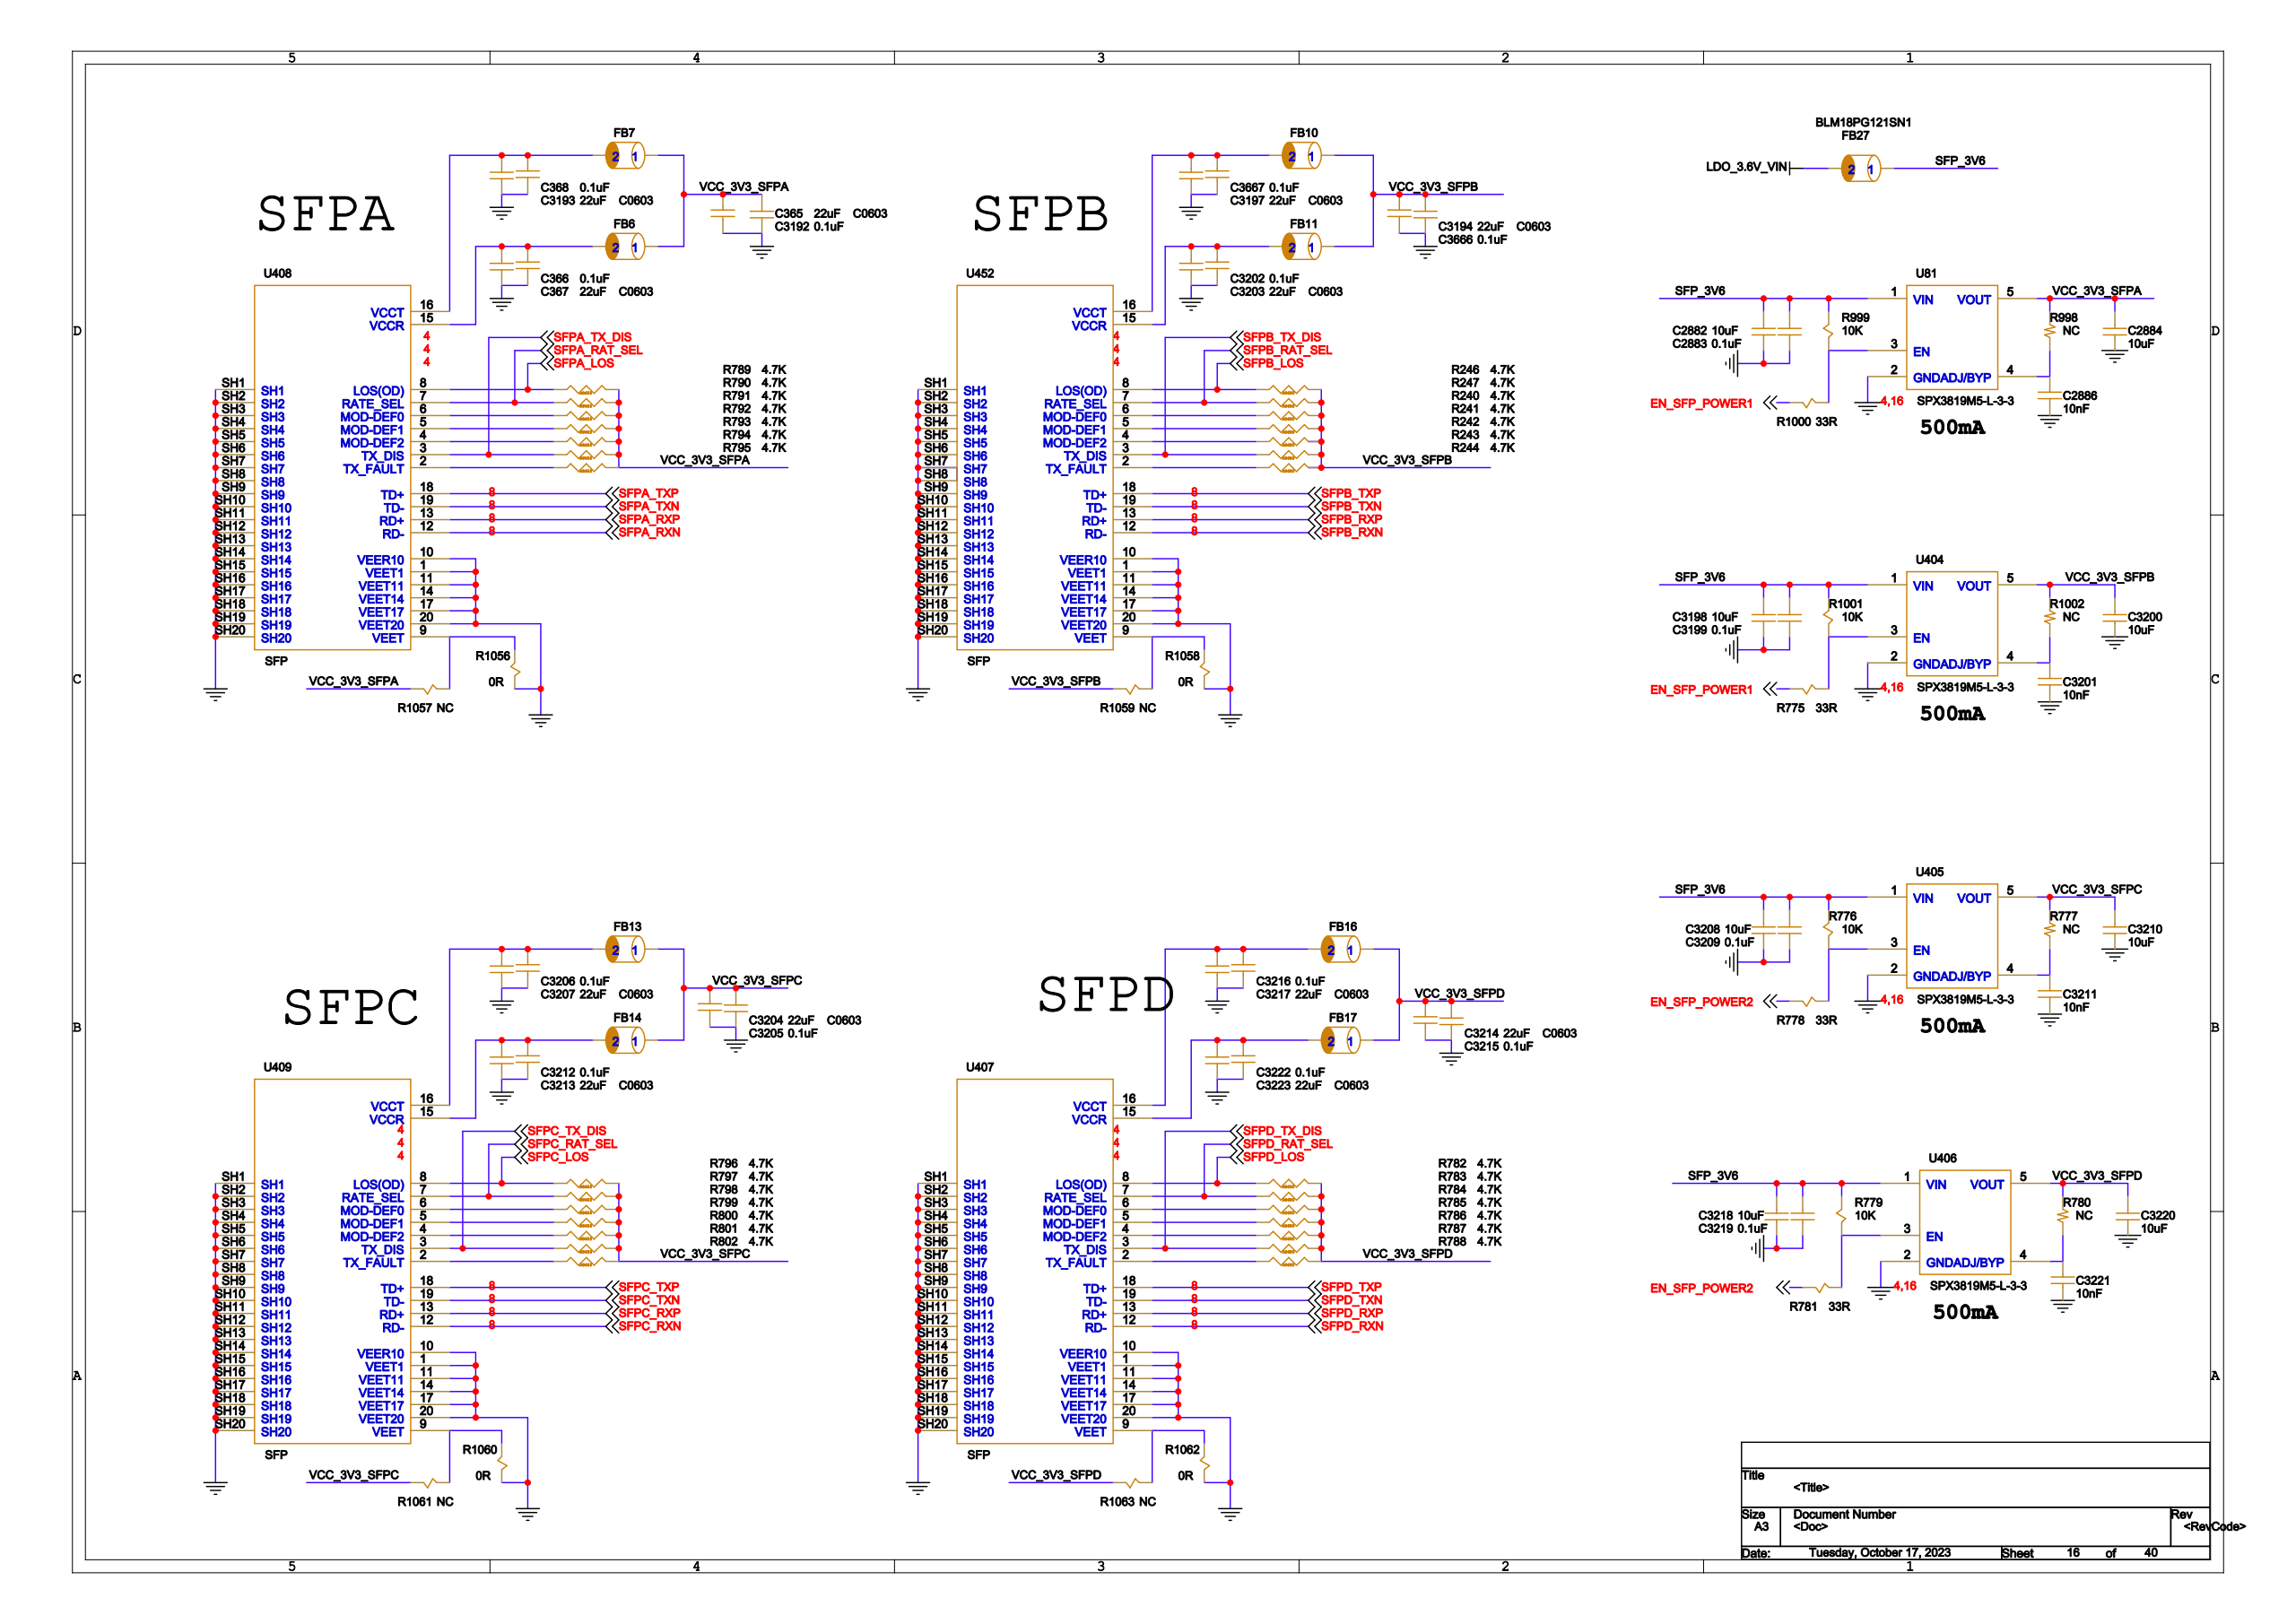Circuit board | Cadence Allegro | 1793 parts | 1223 nets | one sheet of the schematic
Parts on this sheet (reference | value | footprint):
C365 | 22uF | C0603
C366 | 0.1uF | C0402
C367 | 22uF | C0603
C368 | 0.1uF | C0402
C2882 | 10uF | C0402
C2883 | 0.1uF | C0402
C2884 | 10uF | C0402
C2886 | 10nF | C0402
C3192 | 0.1uF | C0402
C3193 | 22uF | C0603
C3194 | 22uF | C0603
C3197 | 22uF | C0603
C3198 | 10uF | C0402
C3199 | 0.1uF | C0402
C3200 | 10uF | C0402
C3201 | 10nF | C0402
C3202 | 0.1uF | C0402
C3203 | 22uF | C0603
C3204 | 22uF | C0603
C3205 | 0.1uF | C0402
C3206 | 0.1uF | C0402
C3207 | 22uF | C0603
C3208 | 10uF | C0402
C3209 | 0.1uF | C0402
C3210 | 10uF | C0402
C3211 | 10nF | C0402
C3212 | 0.1uF | C0402
C3213 | 22uF | C0603
C3214 | 22uF | C0603
C3215 | 0.1uF | C0402
C3216 | 0.1uF | C0402
C3217 | 22uF | C0603
C3218 | 10uF | C0402
C3219 | 0.1uF | C0402
C3220 | 10uF | C0402
C3221 | 10nF | C0402
C3222 | 0.1uF | C0402
C3223 | 22uF | C0603
C3666 | 0.1uF | C0402
C3667 | 0.1uF | C0402
FB6 | BLM18PG121SN1 | FB0603
FB7 | BLM18PG121SN1 | FB0603
FB10 | BLM18PG121SN1 | FB0603
FB11 | BLM18PG121SN1 | FB0603
FB13 | BLM18PG121SN1 | FB0603
FB14 | BLM18PG121SN1 | FB0603
FB16 | BLM18PG121SN1 | FB0603
FB17 | BLM18PG121SN1 | FB0603
FB27 | BLM18PG121SN1 | FB0603
R240 | 4.7K | R0402
R241 | 4.7K | R0402
R242 | 4.7K | R0402
R243 | 4.7K | R0402
R244 | 4.7K | R0402
R246 | 4.7K | R0402
R247 | 4.7K | R0402
R775 | 33R | R0402
R776 | 10K | R0402
R777 | NC | R0402
R778 | 33R | R0402
R779 | 10K | R0402
R780 | NC | R0402
R781 | 33R | R0402
R782 | 4.7K | R0402
R783 | 4.7K | R0402
R784 | 4.7K | R0402
R785 | 4.7K | R0402
R786 | 4.7K | R0402
R787 | 4.7K | R0402
R788 | 4.7K | R0402
R789 | 4.7K | R0402
R790 | 4.7K | R0402
R791 | 4.7K | R0402
R792 | 4.7K | R0402
R793 | 4.7K | R0402
R794 | 4.7K | R0402
R795 | 4.7K | R0402
R796 | 4.7K | R0402
R797 | 4.7K | R0402
R798 | 4.7K | R0402
R799 | 4.7K | R0402
R800 | 4.7K | R0402
R801 | 4.7K | R0402
R802 | 4.7K | R0402
R998 | NC | R0402
R999 | 10K | R0402
R1000 | 33R | R0402
R1001 | 10K | R0402
R1002 | NC | R0402
R1056 | 0R | R0402
R1057 | NC | R0402
R1058 | 0R | R0402
R1059 | NC | R0402
R1060 | 0R | R0402
R1061 | NC | R0402
R1062 | 0R | R0402
R1063 | NC | R0402
U81 | SPX3819M5-L-3-3 | SOT-23-5
U404 | SPX3819M5-L-3-3 | SOT-23-5
U405 | SPX3819M5-L-3-3 | SOT-23-5
U406 | SPX3819M5-L-3-3 | SOT-23-5
U407 | SFP | MOL_74441-0001_CAGE_PFIT
U408 | SFP | MOL_74441-0001_CAGE_PFIT
U409 | SFP | MOL_74441-0001_CAGE_PFIT
U452 | SFP | MOL_74441-0001_CAGE_PFIT
Nets of these parts (net: part-pin ...):
GND: C365-2 C366-1 C367-2 C368-1 C2882-1 C2883-1 C2884-1 C2886-2 C3192-1 C3193-2 C3194-2 C3197-2 C3198-1 C3199-1 C3200-1 C3201-2 C3202-1 C3203-2 C3204-2 C3205-1 C3206-1 C3207-2 C3208-1 C3209-1 C3210-1 C3211-2 C3212-1 C3213-2 C3214-2 C3215-1 C3216-1 C3217-2 C3218-1 C3219-1 C3220-1 C3221-2 C3222-1 C3223-2 C3666-1 C3667-1 R1056-2 R1058-2 R1060-2 R1062-2 U81-2 U404-2 U405-2 U406-2 U407-1 U407-10 U407-11 U407-14 U407-17 U407-20 U407-SH1 U407-SH2 U407-SH3 U407-SH4 U407-SH5 U407-SH6 U407-SH7 U407-SH8 U407-SH9 U407-SH10 U407-SH11 U407-SH12 U407-SH13 U407-SH14 U407-SH15 U407-SH16 U407-SH17 U407-SH18 U407-SH19 U407-SH20 U408-1 U408-10 U408-11 U408-14 U408-17 U408-20 U408-SH1 U408-SH2 U408-SH3 U408-SH4 U408-SH5 U408-SH6 U408-SH7 U408-SH8 U408-SH9 U408-SH10 U408-SH11 U408-SH12 U408-SH13 U408-SH14 U408-SH15 U408-SH16 U408-SH17 U408-SH18 U408-SH19 U408-SH20 U409-1 U409-10 U409-11 U409-14 U409-17 U409-20 U409-SH1 U409-SH2 U409-SH3 U409-SH4 U409-SH5 U409-SH6 U409-SH7 U409-SH8 U409-SH9 U409-SH10 U409-SH11 U409-SH12 U409-SH13 U409-SH14 U409-SH15 U409-SH16 U409-SH17 U409-SH18 U409-SH19 U409-SH20 U452-1 U452-10 U452-11 U452-14 U452-17 U452-20 U452-SH1 U452-SH2 U452-SH3 U452-SH4 U452-SH5 U452-SH6 U452-SH7 U452-SH8 U452-SH9 U452-SH10 U452-SH11 U452-SH12 U452-SH13 U452-SH14 U452-SH15 U452-SH16 U452-SH17 U452-SH18 U452-SH19 U452-SH20
LDO_3.6V_VIN: FB27-2
SFP_3V6: C2882-2 C2883-2 C3198-2 C3199-2 C3208-2 C3209-2 C3218-2 C3219-2 FB27-1 R776-2 R779-2 R999-2 R1001-2 U81-1 U404-1 U405-1 U406-1
VCC_3V3_SFPA: C365-1 C2884-2 C3192-2 FB6-1 FB7-1 R789-2 R790-2 R791-2 R792-2 R793-2 R794-2 R795-2 R998-1 R1057-2 U81-5
VCC_3V3_SFPB: C3194-1 C3200-2 C3666-2 FB10-1 FB11-1 R240-2 R241-2 R242-2 R243-2 R244-2 R246-2 R247-2 R1002-1 R1059-2 U404-5
VCC_3V3_SFPC: C3204-1 C3205-2 C3210-2 FB13-1 FB14-1 R777-1 R796-2 R797-2 R798-2 R799-2 R800-2 R801-2 R802-2 R1061-2 U405-5
VCC_3V3_SFPD: C3214-1 C3215-2 C3220-2 FB16-1 FB17-1 R780-1 R782-2 R783-2 R784-2 R785-2 R786-2 R787-2 R788-2 R1063-2 U406-5
N1523227: C368-2 C3193-1 FB7-2 U408-16
N16981288: C3197-1 C3667-2 FB10-2 U452-16
N16981290: C3202-2 C3203-1 FB11-2 U452-15
N16984632: C3206-2 C3207-1 FB13-2 U409-16
N16984620: C3212-2 C3213-1 FB14-2 U409-15
N16986631: C3216-2 C3217-1 FB16-2 U407-16
N16986629: C3222-2 C3223-1 FB17-2 U407-15
N1522849: C366-2 C367-1 FB6-2 U408-15
N17704771: R1056-1 R1057-1 U408-9
N17705904: R1058-1 R1059-1 U452-9
N17706282: R1060-1 R1061-1 U409-9
N17706684: R1062-1 R1063-1 U407-9
SFPD_LOS: R782-1 U407-8
N17104791: R784-1 U407-6
N17104805: R785-1 U407-5
N17104819: R786-1 U407-4
SFPD_RAT_SEL: R783-1 U407-7
SFPD_RXP: U407-13
SFPD_RXN: U407-12
SFPD_TXP: U407-18
SFPD_TXN: U407-19
SFPD_TX_DIS: R787-1 U407-3
N17104848: R788-1 U407-2
SFPA_LOS: R789-1 U408-8
N17105554: R791-1 U408-6
N17105568: R792-1 U408-5
N17105582: R793-1 U408-4
SFPA_RAT_SEL: R790-1 U408-7
SFPA_RXP: U408-13
SFPA_RXN: U408-12
SFPA_TXP: U408-18
SFPA_TXN: U408-19
SFPA_TX_DIS: R794-1 U408-3
N17105611: R795-1 U408-2
SFPC_LOS: R796-1 U409-8
N17106389: R798-1 U409-6
N17106403: R799-1 U409-5
N17106417: R800-1 U409-4
SFPC_RAT_SEL: R797-1 U409-7
SFPC_RXP: U409-13
SFPC_RXN: U409-12
SFPC_TXP: U409-18
SFPC_TXN: U409-19
SFPC_TX_DIS: R801-1 U409-3
N17106446: R802-1 U409-2
SFPB_LOS: R246-1 U452-8
N661700: R240-1 U452-6
N661736: R241-1 U452-5
N661768: R242-1 U452-4
SFPB_RAT_SEL: R247-1 U452-7
SFPB_RXP: U452-13
SFPB_RXN: U452-12
SFPB_TXP: U452-18
SFPB_TXN: U452-19
SFPB_TX_DIS: R243-1 U452-3
N661880: R244-1 U452-2
N16146404: C2886-1 R998-2 U81-4
N17095883: C3201-1 R1002-2 U404-4
N17096708: C3211-1 R777-2 U405-4
N17097587: C3221-1 R780-2 U406-4
N16146568: R999-1 R1000-1 U81-3
EN_SFP_POWER1: R775-2 R1000-2
N17095879: R775-1 R1001-1 U404-3
N17096704: R776-1 R778-1 U405-3
EN_SFP_POWER2: R778-2 R781-2
N17097583: R779-1 R781-1 U406-3